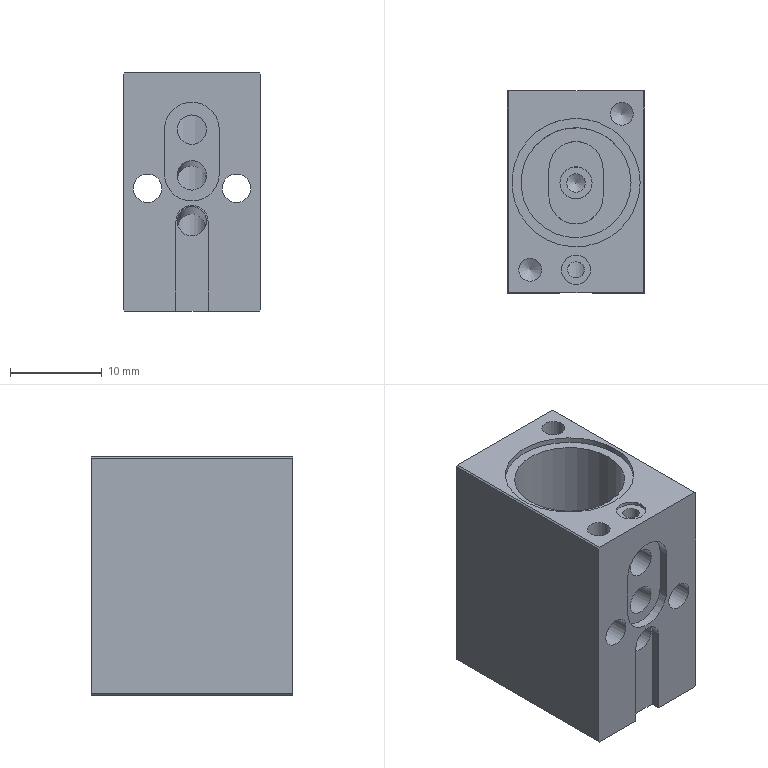NC program | NX | posted with a generic post | part box 15 x 22 x 26 mm
Whole program:
N10 G17 G21 G94 G90
(PLANAR_MILL , TOOL : D50面刀)
N12 T12 M6
N14 G54
N16 G17 G0 G90 X0. Y-61. B0. C0. S3500 M3
N18 G43 Z30. H12
N20 Z2.02
N22 G94 G1 Z0.02 F800.
N24 Y-34.
N26 Y16.
N28 Y43.
N30 Z2.02
N32 G0 Z30.
(PLANAR_MILL_COPY , TOOL : D50面刀)
N34 Y-61.
N36 Z2.
N38 G1 Z0. F400.
N40 Y-34.
N42 Y16.
N44 Y43.
N46 Z2.
N48 G0 Z30.
N50 M5
(ADAPTIVE_MILLING , TOOL : D8开粗)
N52 T13 M6
N54 G54
N56 G17 G0 G90 X19.007 Y-16.963 B0. C0. S5500 M3
N58 G43 Z30. H13
N60 Z-19.
N62 G94 G1 X18.857 Y-16.976 Z-19.937 F3000.
N64 X18.708 Y-16.988 Z-20.308
N66 X18.558 Y-17. Z-20.58
N68 X18.409 Y-17.012 Z-20.8
N70 X18.259 Y-17.024 Z-20.984
N72 X18.11 Y-17.036 Z-21.142
N74 X17.96 Y-17.049 Z-21.28
N76 X17.811 Y-17.061 Z-21.4
N78 X17.661 Y-17.073 Z-21.505
N80 X17.512 Y-17.085 Z-21.598
N82 X17.362 Y-17.097 Z-21.679
N84 X17.213 Y-17.109 Z-21.75
N86 X17.063 Y-17.121 Z-21.81
N88 X16.914 Y-17.134 Z-21.862
N90 X16.764 Y-17.146 Z-21.905
N92 X16.615 Y-17.158 Z-21.939
N94 X16.465 Y-17.17 Z-21.966
N96 X16.316 Y-17.182 Z-21.985
N98 X16.166 Y-17.194 Z-21.996
N100 X16.017 Y-17.206 Z-22.
N102 X14.661 Y-17.317
N104 G3 X14.012 Y-17.743 R0.809
N106 X13.466 Y-19.934 R6.485
N108 X13.212 Y-26.49 R66.401
N110 G2 X13.179 Y-32.052 R316.859
N112 X11.283 Y-35.133 R4.581
N114 X7.426 Y-36.699 R9.099
N116 X1.99 Y-37.144 R34.543
N118 X-8.029 Y-37.179 R356.472
N120 X-11.073 Y-35.328 R4.571
N122 X-12.702 Y-31.358 R9.168
N124 X-13.147 Y-25.802 R35.318
N126 X-13.197 Y-15.422 R693.892
N128 G1 X-13.196 Y13.776
N130 G2 X-11.571 Y16.874 R4.369
N132 X-7.853 Y18.599 R8.451
N134 X-2.367 Y19.133 R29.556
N136 X8.012 Y19.181 R421.599
N138 X11.072 Y17.361 R4.531
N140 X12.68 Y13.523 R8.908
N142 X13.145 Y7.908 R34.05
N144 X13.197 Y-2.891 R711.007
N146 X13.181 Y-15.25 R926.327
N148 X12.727 Y-19.572 R142.497
N150 G3 X12.413 Y-28.169 R102.8
N152 G2 X12.289 Y-30.434 R11.462
N154 X9.475 Y-34.316 R6.17
N156 X5.027 Y-35.898 R11.721
N158 X-1.131 Y-36.348 R43.367
N160 X-5.81 Y-36.363 R78.179
N162 X-10.137 Y-33.713 R6.
N164 X-11.828 Y-29.386 R11.008
N166 X-12.338 Y-23.294 R38.421
N168 X-12.397 Y-14.054 R652.598
N170 G1 Y11.316
N172 G2 X-11.111 Y14.854 R5.682
N174 X-10.434 Y15.785 R4.136
N176 X-8.677 Y16.95 R5.031
N178 X-3.547 Y18.125 R16.802
N180 X4.006 Y18.382 R91.374
N182 X6.281 Y18.303 R13.433
N184 X9.493 Y16.545 R6.058
N186 X10.086 Y16.133 R16.9
N188 G1 X10.948 Y15.163
N190 G2 X11.676 Y13.213 R5.416
N192 X12.31 Y6.894 R35.469
N194 X12.397 Y-6.426 R558.887
N196 X12.358 Y-14.29 R256.673
N198 X11.877 Y-20.385 R446.631
N200 G3 X11.606 Y-27.892 R216.059
N202 G2 X8.221 Y-33.366 R6.978
N204 X3.428 Y-35.054 R12.952
N206 X-4.048 Y-35.515 R42.098
N208 X-9.244 Y-32.359 R6.85
N210 X-11.026 Y-27.551 R12.485
N212 X-11.534 Y-21.217 R42.943
N214 X-11.595 Y-13.413 R615.746
N216 G1 X-11.65 Y-12.879
N218 Y12.851
N220 G2 X-10.434 Y15.785 R4.323
N222 X-7.349 Y17.15 R4.29
N224 G3 X-3.62 Y17.329 R41.85
N226 G2 X3.935 Y17.539 R91.272
N228 X5.872 Y17.157 R8.704
N230 X8.152 Y17.072 R17.123
N232 X9.559 Y16.505 R4.648
N234 G3 X7.351 Y17.15 R4.314
N236 G1 X-6.428
N238 G2 X-7.005 Y18.505 R0.8
N240 X-6.558 Y18.754 Z-21.967 R1.036
N242 G1 X-5.566 Y19.111 Z-21.9
N244 X-4.199 Y19.603 F15000.
N246 X-4.065 Y19.637
N248 X-3.928 Y19.651
N250 X10.466
N252 G2 X12.136 Y18.374 R1.731
N254 G1 X12.483 Y17.097
N256 G2 X12.471 Y16.636 R0.813
N258 G1 X12.422 Y16.489
N260 X11.929 Y14.997 Z-22. F3000.
N262 X11.746 Y14.453
N264 G3 X11.568 Y13.681 R2.215
N266 G1 X11.65 Y12.879
N268 Y-12.851
N270 G3 X10.956 Y-23.053 R297.803
N272 G2 X10.793 Y-26.73 R61.381
N274 X6.846 Y-32.597 R7.738
N276 X1.856 Y-34.25 R14.385
N278 X-2.624 Y-34.588 R22.441
N280 X-8.432 Y-31.017 R7.384
N282 X-10.214 Y-26.005 R13.583
N284 X-10.732 Y-19.371 R46.31
N286 G1 X-10.792 Y-15.53
N288 G3 X-10.921 Y-15.196 R3.884
N290 X-11.628 Y-14.9 R0.801
N292 G1 X-13.191 Y-15.07 Z-21.9
N294 X-14.385 Y-15.198 F15000.
N296 X-14.589 Y-15.186
N298 X-14.791 Y-15.161
N300 G2 X-14.9 Y-13.641 R0.8
N302 G1 X-13.616 Y-13.125
N304 X-13.102 Y-12.914 Z-21.935 F3000.
N306 X-12.581 Y-12.717 Z-21.971
N308 G2 X-12.129 Y-12.739 Z-22. R0.833
N310 X-11.595 Y-13.413 R0.801
N312 G3 X-10.837 Y-15.302 R3.88
N314 G2 X-10.443 Y-17.196 R6.14
N316 X-10.074 Y-22.882 R845.805
N318 G3 X-9.028 Y-28.286 R21.086
N320 X-6.195 Y-32.302 R8.471
N322 X-1.819 Y-33.79 R8.338
N324 X5.333 Y-32.615 R15.022
N326 X9.908 Y-26.933 R7.897
N328 X10.48 Y-22.233 R30.747
N330 G1 X10.998 Y-15.131
N332 G2 X11.333 Y-14.439 R3.786
N334 G1 X11.57 Y-13.661
N336 G2 X10.918 Y-15.208 R4.785
N338 G3 X10.173 Y-17.945 R9.352
N340 X9.57 Y-23.517 R127.747
N342 G2 X8.658 Y-27.416 R13.216
N344 X4.086 Y-31.76 R8.531
N346 X-2.195 Y-32.587 R11.311
N348 X-7.21 Y-28.985 R7.486
N350 X-8.944 Y-23.963 R14.179
N352 X-9.529 Y-18.559 R69.222
N354 G3 X-9.891 Y-16.393 R9.77
N356 X-10.435 Y-15.784 R2.724
N358 G1 X-10.894 Y-15.229
N360 G3 X-9.972 Y-16.225 R6.624
N362 G2 X-9.338 Y-17.833 R3.93
N364 X-8.723 Y-22.057 R59.276
N366 G3 X-7.516 Y-26.936 R19.134
N368 X-4.047 Y-30.944 R7.906
N370 X2.083 Y-31.632 R8.844
N372 X8.34 Y-25.905 R8.322
N374 X9.252 Y-21.323 R23.862
N376 G2 X9.97 Y-16.818 R38.253
N378 X10.332 Y-15.882 R2.45
N380 G1 X10.95 Y-15.157
N382 G2 X10.098 Y-16.105 R6.886
N384 G3 X9.144 Y-18.275 R6.004
N386 X8.27 Y-22.598 R70.776
N388 G2 X6.811 Y-26.704 R12.491
N390 X-1.158 Y-30.429 R7.891
N392 X-5.738 Y-27.279 R7.098
N394 X-7.586 Y-22.669 R13.658
N396 G3 X-8.431 Y-18.505 R723.672
N398 X-9.036 Y-16.859 R5.261
N400 X-9.633 Y-16.466 R1.751
N402 G1 X-10.033 Y-16.175
N404 G3 X-9.252 Y-16.671 R3.922
N406 G2 X-8.619 Y-17.38 R1.523
N408 X-7.662 Y-20.269 R12.083
N410 G3 X-6.447 Y-24.534 R29.825
N412 X-3.81 Y-28.212 R8.465
N414 X4.983 Y-27.5 R6.744
N416 X7.308 Y-23.542 R9.808
N418 X8.4 Y-19.341 R57.072
N420 G2 X9.357 Y-16.714 R10.449
N422 X9.82 Y-16.337 R1.609
N424 G1 X10.222 Y-15.976
N426 G2 X9.316 Y-16.665 R4.468
N428 G3 X8.168 Y-18.436 R4.611
N430 X6.9 Y-22.141 R62.
N432 G2 X4.893 Y-25.8 R10.439
N434 X-0.156 Y-27.799 R5.82
N436 X-4.235 Y-25.362 R6.397
N438 X-6.307 Y-21.387 R13.342
N440 G3 X-7.53 Y-18.122 R35.488
N442 X-8.198 Y-17.115 R2.961
N444 X-8.982 Y-16.815 R2.761
N446 G1 X-9.194 Y-16.702
N448 G3 X-8.224 Y-17.066 R4.709
N450 G2 X-7.121 Y-18.415 R3.471
N452 X-5.71 Y-21.623 R45.98
N454 G3 X-3.657 Y-24.914 R10.933
N456 X3.358 Y-25.512 R5.274
N458 X6.022 Y-22.218 R8.774
N460 X7.522 Y-18.792 R89.769
N462 G2 X8.647 Y-16.983 R6.207
N464 X9.478 Y-16.563 R9.69
N466 G1 X8.43 Y-17.052
N468 G3 X7.016 Y-18.732 R5.233
N470 G2 X5.317 Y-21.74 R111.737
N472 X2.976 Y-24.084 R6.494
N474 X-1.354 Y-23.993 R4.725
N476 X-4.392 Y-21.194 R8.525
N478 G1 X-6.231 Y-18.37
N480 G3 X-7.221 Y-17.26 R4.947
N482 X-7.563 Y-17.143 R2.096
N484 G1 X-8.28 Y-17.044
N486 G2 X-7.265 Y-17.195 R7.725
N488 X-5.903 Y-18.375 R4.056
N490 G3 X-3.836 Y-21.058 R132.827
N492 X-1.594 Y-22.834 R6.201
N494 X2.734 Y-22.415 R4.948
N496 X5.531 Y-19.808 R9.767
N498 G2 X7.38 Y-17.533 R21.781
N500 X8.019 Y-17.096 R1.508
N502 G1 X8.716 Y-16.913
N504 G3 X7.554 Y-17.211 R15.357
N506 X5.882 Y-18.507 R6.278
N508 G2 X3.666 Y-20.499 R16.448
N510 X-0.424 Y-20.984 R4.752
N512 X-3.666 Y-19.09 R9.536
N514 G3 X-5.9 Y-17.312 R22.862
N516 X-6.359 Y-17.146 R1.189
N518 G1 X-7.499 Y-17.145
N520 X-6.18 Y-17.148
N522 G2 X-4.491 Y-18.005 R5.064
N524 G3 X-1.896 Y-19.637 R19.188
N526 X2.48 Y-19.695 R5.526
N528 X5.458 Y-17.998 R14.249
N530 G2 X6.872 Y-17.18 R8.237
N532 X7.797 Y-17.125 R11.301
N534 G1 X6.632 Y-17.162
N536 G3 X4.865 Y-17.779 R7.422
N538 G2 X2.132 Y-18.68 R9.551
N540 X-1.973 Y-18.031 R8.401
N542 G1 X-4.042 Y-17.171
N544 X-4.195 Y-17.146
N546 X-6.295
N548 X-3.85 Y-17.162
N550 G2 X-1.319 Y-17.768 R40.229
N552 G3 X3.365 Y-17.574 R9.295
N554 G1 X4.925 Y-17.149
N556 X6.785 Y-17.15
N558 X-4.015 Y-17.146
N560 G3 X-4.811 Y-18.094 R0.808
N562 G1 X-4.633 Y-19.111
N564 X-4.608 Y-19.259 Z-21.996
N566 X-4.582 Y-19.406 Z-21.985
N568 X-4.556 Y-19.554 Z-21.966
N570 X-4.53 Y-19.702 Z-21.939
N572 X-4.504 Y-19.85 Z-21.905
N574 X-4.478 Y-19.997 Z-21.862
N576 X-4.452 Y-20.145 Z-21.81
N578 X-4.427 Y-20.293 Z-21.75
N580 X-4.401 Y-20.441 Z-21.679
N582 X-4.375 Y-20.588 Z-21.598
N584 X-4.349 Y-20.736 Z-21.505
N586 X-4.323 Y-20.884 Z-21.4
N588 X-4.297 Y-21.032 Z-21.28
N590 X-4.271 Y-21.179 Z-21.142
N592 X-4.246 Y-21.327 Z-20.984
N594 X-4.22 Y-21.475 Z-20.8
N596 X-4.194 Y-21.623 Z-20.58
N598 X-4.168 Y-21.77 Z-20.308
N600 X-4.142 Y-21.918 Z-19.937
N602 X-4.116 Y-22.066 Z-19.
N604 G0 Z30.
N606 M5
(PLANAR_MILL_1 , TOOL : D8精光)
N608 T01 M6
N610 G54
N612 G17 G0 G90 X7.007 Y19. B0. C0. S5000 M3
N614 G43 Z30. H1
N616 Z-20.
N618 G94 G1 Z-22. F600.
N620 X10.179 Y15.828
N622 X10.328 Y15.678
N624 G2 X11.5 Y12.85 R4.
N626 G1 Y-12.85
N628 G2 X10.328 Y-15.678 R4.
N630 G1 X10.178 Y-15.828
N632 G2 X7.35 Y-17. R4.
N634 G1 X-7.35
N636 G2 X-10.178 Y-15.828 R4.
N638 G1 X-10.328 Y-15.678
N640 G2 X-11.5 Y-12.85 R4.
N642 G1 Y12.85
N644 G2 X-10.328 Y15.678 R4.
N646 G1 X-10.178 Y15.828
N648 G2 X-7.35 Y17. R4.
N650 G1 X7.349
N652 X11.833
N654 Z-20.
N656 G0 Z30.
N658 X7.007 Y19.
N660 Z-20.
N662 G1 Z-22.
N664 X10.179 Y15.828
N666 X10.328 Y15.678
N668 G2 X11.5 Y12.85 R4.
N670 G1 Y-12.85
N672 G2 X10.328 Y-15.678 R4.
N674 G1 X10.178 Y-15.828
N676 G2 X7.35 Y-17. R4.
N678 G1 X-7.35
N680 G2 X-10.178 Y-15.828 R4.
N682 G1 X-10.328 Y-15.678
N684 G2 X-11.5 Y-12.85 R4.
N686 G1 Y12.85
N688 G2 X-10.328 Y15.678 R4.
N690 G1 X-10.178 Y15.828
N692 G2 X-7.35 Y17. R4.
N694 G1 X7.349
N696 X11.833
N698 Z-20.
N700 G0 Z30.
N702 M5
(PLANAR_MILL_2 , TOOL : D3开粗)
N704 T14 M6
N706 G54
N708 G17 G0 G90 X-1.134 Y1.188 B0. C0. S4500 M3
N710 G43 Z30. H14
N712 Z0.2
N714 G94 G1 X-1.026 Y0.989 Z0.198 F800.
N716 X-0.307 Y0.6 Z0.191
N718 X0.276 Z0.186
N720 X0.996 Y0.989 Z0.179
N722 X1.385 Y1.709 Z0.172
N724 Y7.091 Z0.125
N726 X0.996 Y7.811 Z0.117
N728 X0.276 Y8.2 Z0.11
N730 X-0.307 Z0.105
N732 X-1.026 Y7.811 Z0.098
N734 X-1.415 Y7.091 Z0.091
N736 Y1.709 Z0.044
N738 X-1.026 Y0.989 Z0.037
N740 X-0.307 Y0.6 Z0.03
N742 X0.276 Z0.025
N744 X0.996 Y0.989 Z0.017
N746 X1.385 Y1.709 Z0.01
N748 Y7.091 Z-0.037
N750 X0.996 Y7.811 Z-0.044
N752 X0.276 Y8.2 Z-0.051
N754 X-0.307 Z-0.056
N756 X-1.026 Y7.811 Z-0.063
N758 X-1.415 Y7.091 Z-0.07
N760 Y1.709 Z-0.117
N762 X-1.026 Y0.989 Z-0.124
N764 X-0.307 Y0.6 Z-0.132
N766 X0.276 Z-0.137
N768 X0.996 Y0.989 Z-0.144
N770 X1.385 Y1.709 Z-0.151
N772 Y7.091 Z-0.198
N774 X0.996 Y7.811 Z-0.205
N776 X0.276 Y8.2 Z-0.212
N778 X-0.307 Z-0.217
N780 X-1.026 Y7.811 Z-0.224
N782 X-1.415 Y7.091 Z-0.232
N784 Y1.709 Z-0.279
N786 X-1.026 Y0.989 Z-0.286
N788 X-0.307 Y0.6 Z-0.293
N790 X0.276 Z-0.298
N792 X0.996 Y0.989 Z-0.305
N794 X1.385 Y1.709 Z-0.312
N796 Y7.091 Z-0.359
N798 X0.996 Y7.811 Z-0.366
N800 X0.276 Y8.2 Z-0.373
N802 X-0.307 Z-0.379
N804 X-1.026 Y7.811 Z-0.386
N806 X-1.415 Y7.091 Z-0.393
N808 Y1.709 Z-0.44
N810 X-1.026 Y0.989 Z-0.447
N812 X-0.307 Y0.6 Z-0.454
N814 X0.276 Z-0.459
N816 X0.996 Y0.989 Z-0.466
N818 X1.385 Y1.709 Z-0.473
N820 Y7.091 Z-0.52
N822 X0.996 Y7.811 Z-0.528
N824 X0.276 Y8.2 Z-0.535
N826 X-0.307 Z-0.54
N828 X-1.026 Y7.811 Z-0.547
N830 X-1.415 Y7.091 Z-0.554
N832 Y1.709 Z-0.601
N834 X-1.026 Y0.989 Z-0.608
N836 X-0.307 Y0.6 Z-0.615
N838 X0.276 Z-0.62
N840 X0.996 Y0.989 Z-0.628
N842 X1.385 Y1.709 Z-0.635
N844 Y7.091 Z-0.682
N846 X0.996 Y7.811 Z-0.689
N848 X0.276 Y8.2 Z-0.696
N850 X-0.307 Z-0.701
N852 X-1.026 Y7.811 Z-0.708
N854 X-1.415 Y7.091 Z-0.715
N856 Y1.709 Z-0.762
N858 X-1.026 Y0.989 Z-0.769
N860 X-0.307 Y0.6 Z-0.777
N862 X0.276 Z-0.782
N864 X0.996 Y0.989 Z-0.789
N866 X1.385 Y1.709 Z-0.796
N868 Y7.091 Z-0.843
N870 X0.996 Y7.811 Z-0.85
N872 X0.276 Y8.2 Z-0.857
N874 X-0.307 Z-0.862
N876 X-1.026 Y7.811 Z-0.869
N878 X-1.415 Y7.091 Z-0.877
N880 Y4.4 Z-0.9
N882 Y2.
N884 G3 X-0.015 Y0.6 R1.4
N886 X1.385 Y2. R1.4
N888 G1 Y6.8
N890 G3 X-0.015 Y8.2 R1.4
N892 X-1.415 Y6.8 R1.4
N894 G1 Y4.4
N896 Z-0.7
N898 G0 Z30.
(PLANAR_MILL_3 , TOOL : D3开粗)
N900 X0.15 Y-16.5
N902 Z1.7
N904 G1 Z-0.3
N906 Y-13.
N908 Y-3.2
N910 G3 X0. Y-3.05 R0.15
N912 X-0.15 Y-3.2 R0.15
N914 G1 Y-13.
N916 Y-16.5
N918 Z1.7
N920 G0 Z30.
N922 X0.15
N924 Z1.4
N926 G1 Z-0.6
N928 Y-13.
N930 Y-3.2
N932 G3 X0. Y-3.05 R0.15
N934 X-0.15 Y-3.2 R0.15
N936 G1 Y-13.
N938 Y-16.5
N940 Z1.4
N942 G0 Z30.
N944 X0.15
N946 Z1.1
N948 G1 Z-0.9
N950 Y-13.
N952 Y-3.2
N954 G3 X0. Y-3.05 R0.15
N956 X-0.15 Y-3.2 R0.15
N958 G1 Y-13.
N960 Y-16.5
N962 Z1.1
N964 G0 Z30.
N966 M5
(DRILLING , TOOL : D4点钻)
N968 T02 M6
N970 G54
N972 G17 G0 G90 X4.85 Y0.4 B0. C0. S3000 M3
N974 G43 Z30. H2
N976 G94 G81 G98 Z-1.6 F200. R3.
N978 X-4.85
N980 G80
N982 G0 X-4.85 Y0.4 Z30.
(DRILLING_COPY , TOOL : D4点钻)
N984 X-0.015 Y6.8
N986 G81 Z-2.7 F200. R2.
N988 G80
N990 G0 X-0.015 Y6.8 Z30.
N992 M5
(DRILLING_COPY_1 , TOOL : D3.1钻头)
N994 T03 M6
N996 G54
N998 G17 G0 G90 X4.85 Y0.4 B0. C0. S3000 M3
N1000 G43 Z30. H3
N1002 G94 G83 G98 Z-25. F200. Q2. R3.
N1004 X-4.85
N1006 G80
N1008 G0 X-4.85 Y0.4 Z30.
N1010 M5
(DRILLING_COPY_COPY , TOOL : D3.2钻头)
N1012 T04 M6
N1014 G54
N1016 G17 G0 G90 X-0.015 Y6.8 B0. C0. S3000 M3
N1018 G43 Z30. H4
N1020 G94 G81 G98 Z-9. F200. R2.
N1022 G80
N1024 G0 X-0.015 Y6.8 Z30.
N1026 M5
N1028 M2